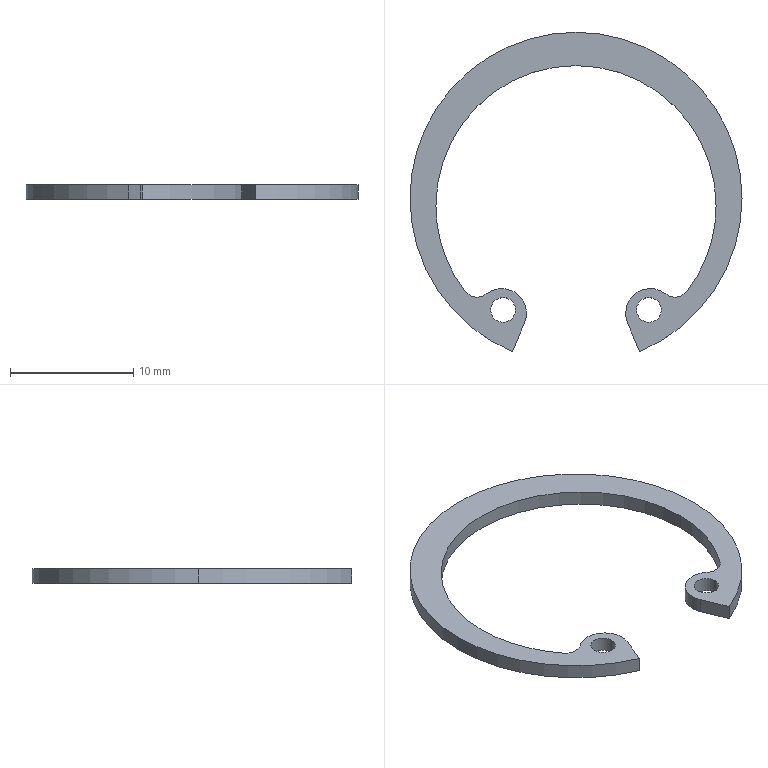Part | SolidWorks | features Extrusion 1 | 1 solid | 19 faces | box 26.9 x 25.876 x 1.2 mm | volume 193.596 mm3 | cylinder 15 | plane 4 | commonest cylinder face diameters 2 x4 4 x3 22.7 x3 26.9 x3 2.4 x2
STEP:
#1=CARTESIAN_POINT('',(4.909,-9.04,1.2));
#2=VERTEX_POINT('',#1);
#3=CARTESIAN_POINT('',(6.909,-9.04,1.2));
#4=VERTEX_POINT('',#3);
#5=CARTESIAN_POINT('',(5.909,-9.04,1.2));
#6=DIRECTION('',(0.,0.,1.));
#7=DIRECTION('',(-1.,0.,0.));
#8=AXIS2_PLACEMENT_3D('',#5,#6,#7);
#9=CIRCLE('',#8,1.);
#10=EDGE_CURVE('',#2,#4,#9,.T.);
#11=ORIENTED_EDGE('',*,*,#10,.T.);
#12=CARTESIAN_POINT('',(6.909,-9.04,0.));
#13=VERTEX_POINT('',#12);
#14=CARTESIAN_POINT('',(6.909,-9.04,1.2));
#15=DIRECTION('',(0.,0.,-1.));
#16=VECTOR('',#15,1000.);
#17=LINE('',#14,#16);
#18=EDGE_CURVE('',#4,#13,#17,.T.);
#19=ORIENTED_EDGE('',*,*,#18,.T.);
#20=CARTESIAN_POINT('',(4.909,-9.04,0.));
#21=VERTEX_POINT('',#20);
#22=CARTESIAN_POINT('',(5.909,-9.04,0.));
#23=DIRECTION('',(0.,0.,1.));
#24=DIRECTION('',(-1.,0.,0.));
#25=AXIS2_PLACEMENT_3D('',#22,#23,#24);
#26=CIRCLE('',#25,1.);
#27=EDGE_CURVE('',#21,#13,#26,.T.);
#28=ORIENTED_EDGE('',*,*,#27,.F.);
#29=CARTESIAN_POINT('',(4.909,-9.04,1.2));
#30=DIRECTION('',(0.,0.,-1.));
#31=VECTOR('',#30,1000.);
#32=LINE('',#29,#31);
#33=EDGE_CURVE('',#2,#21,#32,.T.);
#34=ORIENTED_EDGE('',*,*,#33,.F.);
#35=EDGE_LOOP('',(#11,#19,#28,#34));
#36=FACE_OUTER_BOUND('',#35,.T.);
#37=CARTESIAN_POINT('',(5.909,-9.04,1.2));
#38=DIRECTION('',(0.,0.,-1.));
#39=DIRECTION('',(-1.,0.,0.));
#40=AXIS2_PLACEMENT_3D('',#37,#38,#39);
#41=CYLINDRICAL_SURFACE('',#40,1.);
#42=ADVANCED_FACE('',(#36),#41,.F.);
#43=CARTESIAN_POINT('',(-6.909,-9.04,1.2));
#44=VERTEX_POINT('',#43);
#45=CARTESIAN_POINT('',(-4.909,-9.04,1.2));
#46=VERTEX_POINT('',#45);
#47=CARTESIAN_POINT('',(-5.909,-9.04,1.2));
#48=DIRECTION('',(0.,0.,1.));
#49=DIRECTION('',(1.,0.,0.));
#50=AXIS2_PLACEMENT_3D('',#47,#48,#49);
#51=CIRCLE('',#50,1.);
#52=EDGE_CURVE('',#44,#46,#51,.T.);
#53=ORIENTED_EDGE('',*,*,#52,.T.);
#54=CARTESIAN_POINT('',(-4.909,-9.04,0.));
#55=VERTEX_POINT('',#54);
#56=CARTESIAN_POINT('',(-4.909,-9.04,1.2));
#57=DIRECTION('',(0.,0.,-1.));
#58=VECTOR('',#57,1000.);
#59=LINE('',#56,#58);
#60=EDGE_CURVE('',#46,#55,#59,.T.);
#61=ORIENTED_EDGE('',*,*,#60,.T.);
#62=CARTESIAN_POINT('',(-6.909,-9.04,0.));
#63=VERTEX_POINT('',#62);
#64=CARTESIAN_POINT('',(-5.909,-9.04,0.));
#65=DIRECTION('',(0.,0.,1.));
#66=DIRECTION('',(1.,0.,0.));
#67=AXIS2_PLACEMENT_3D('',#64,#65,#66);
#68=CIRCLE('',#67,1.);
#69=EDGE_CURVE('',#63,#55,#68,.T.);
#70=ORIENTED_EDGE('',*,*,#69,.F.);
#71=CARTESIAN_POINT('',(-6.909,-9.04,1.2));
#72=DIRECTION('',(0.,0.,-1.));
#73=VECTOR('',#72,1000.);
#74=LINE('',#71,#73);
#75=EDGE_CURVE('',#44,#63,#74,.T.);
#76=ORIENTED_EDGE('',*,*,#75,.F.);
#77=EDGE_LOOP('',(#53,#61,#70,#76));
#78=FACE_OUTER_BOUND('',#77,.T.);
#79=CARTESIAN_POINT('',(-5.909,-9.04,1.2));
#80=DIRECTION('',(0.,0.,-1.));
#81=DIRECTION('',(-1.,0.,0.));
#82=AXIS2_PLACEMENT_3D('',#79,#80,#81);
#83=CYLINDRICAL_SURFACE('',#82,1.);
#84=ADVANCED_FACE('',(#78),#83,.F.);
#85=CARTESIAN_POINT('',(13.45,0.,1.2));
#86=VERTEX_POINT('',#85);
#87=CARTESIAN_POINT('',(-13.45,0.,1.2));
#88=VERTEX_POINT('',#87);
#89=CARTESIAN_POINT('',(0.,0.,1.2));
#90=DIRECTION('',(0.,0.,1.));
#91=DIRECTION('',(1.,0.,0.));
#92=AXIS2_PLACEMENT_3D('',#89,#90,#91);
#93=CIRCLE('',#92,13.45);
#94=EDGE_CURVE('',#86,#88,#93,.T.);
#95=ORIENTED_EDGE('',*,*,#94,.F.);
#96=CARTESIAN_POINT('',(13.45,0.,0.));
#97=VERTEX_POINT('',#96);
#98=CARTESIAN_POINT('',(13.45,0.,1.2));
#99=DIRECTION('',(0.,0.,-1.));
#100=VECTOR('',#99,1000.);
#101=LINE('',#98,#100);
#102=EDGE_CURVE('',#86,#97,#101,.T.);
#103=ORIENTED_EDGE('',*,*,#102,.T.);
#104=CARTESIAN_POINT('',(-13.45,0.,0.));
#105=VERTEX_POINT('',#104);
#106=CARTESIAN_POINT('',(0.,0.,0.));
#107=DIRECTION('',(0.,0.,1.));
#108=DIRECTION('',(1.,0.,0.));
#109=AXIS2_PLACEMENT_3D('',#106,#107,#108);
#110=CIRCLE('',#109,13.45);
#111=EDGE_CURVE('',#97,#105,#110,.T.);
#112=ORIENTED_EDGE('',*,*,#111,.T.);
#113=CARTESIAN_POINT('',(-13.45,0.,1.2));
#114=DIRECTION('',(0.,0.,-1.));
#115=VECTOR('',#114,1000.);
#116=LINE('',#113,#115);
#117=EDGE_CURVE('',#88,#105,#116,.T.);
#118=ORIENTED_EDGE('',*,*,#117,.F.);
#119=EDGE_LOOP('',(#95,#103,#112,#118));
#120=FACE_OUTER_BOUND('',#119,.T.);
#121=CARTESIAN_POINT('',(0.,0.,1.2));
#122=DIRECTION('',(0.,0.,-1.));
#123=DIRECTION('',(-1.,0.,0.));
#124=AXIS2_PLACEMENT_3D('',#121,#122,#123);
#125=CYLINDRICAL_SURFACE('',#124,13.45);
#126=ADVANCED_FACE('',(#120),#125,.T.);
#127=CARTESIAN_POINT('',(-5.147,-12.426,1.2));
#128=VERTEX_POINT('',#127);
#129=CARTESIAN_POINT('',(0.,0.,1.2));
#130=DIRECTION('',(0.,0.,1.));
#131=DIRECTION('',(1.,0.,0.));
#132=AXIS2_PLACEMENT_3D('',#129,#130,#131);
#133=CIRCLE('',#132,13.45);
#134=EDGE_CURVE('',#88,#128,#133,.T.);
#135=ORIENTED_EDGE('',*,*,#134,.F.);
#136=ORIENTED_EDGE('',*,*,#117,.T.);
#137=CARTESIAN_POINT('',(-5.147,-12.426,0.));
#138=VERTEX_POINT('',#137);
#139=CARTESIAN_POINT('',(0.,0.,0.));
#140=DIRECTION('',(0.,0.,1.));
#141=DIRECTION('',(1.,0.,0.));
#142=AXIS2_PLACEMENT_3D('',#139,#140,#141);
#143=CIRCLE('',#142,13.45);
#144=EDGE_CURVE('',#105,#138,#143,.T.);
#145=ORIENTED_EDGE('',*,*,#144,.T.);
#146=CARTESIAN_POINT('',(-5.147,-12.426,1.2));
#147=DIRECTION('',(0.,0.,-1.));
#148=VECTOR('',#147,1000.);
#149=LINE('',#146,#148);
#150=EDGE_CURVE('',#128,#138,#149,.T.);
#151=ORIENTED_EDGE('',*,*,#150,.F.);
#152=EDGE_LOOP('',(#135,#136,#145,#151));
#153=FACE_OUTER_BOUND('',#152,.T.);
#154=CARTESIAN_POINT('',(0.,0.,1.2));
#155=DIRECTION('',(0.,0.,-1.));
#156=DIRECTION('',(-1.,0.,0.));
#157=AXIS2_PLACEMENT_3D('',#154,#155,#156);
#158=CYLINDRICAL_SURFACE('',#157,13.45);
#159=ADVANCED_FACE('',(#153),#158,.T.);
#160=CARTESIAN_POINT('',(4.022,-9.312,1.2));
#161=VERTEX_POINT('',#160);
#162=CARTESIAN_POINT('',(4.174,-10.078,1.2));
#163=VERTEX_POINT('',#162);
#164=CARTESIAN_POINT('',(6.022,-9.312,1.2));
#165=DIRECTION('',(0.,0.,1.));
#166=DIRECTION('',(-1.,0.,0.));
#167=AXIS2_PLACEMENT_3D('',#164,#165,#166);
#168=CIRCLE('',#167,2.);
#169=EDGE_CURVE('',#161,#163,#168,.T.);
#170=ORIENTED_EDGE('',*,*,#169,.F.);
#171=CARTESIAN_POINT('',(4.022,-9.312,0.));
#172=VERTEX_POINT('',#171);
#173=CARTESIAN_POINT('',(4.022,-9.312,1.2));
#174=DIRECTION('',(0.,0.,-1.));
#175=VECTOR('',#174,1000.);
#176=LINE('',#173,#175);
#177=EDGE_CURVE('',#161,#172,#176,.T.);
#178=ORIENTED_EDGE('',*,*,#177,.T.);
#179=CARTESIAN_POINT('',(4.174,-10.078,0.));
#180=VERTEX_POINT('',#179);
#181=CARTESIAN_POINT('',(6.022,-9.312,0.));
#182=DIRECTION('',(0.,0.,1.));
#183=DIRECTION('',(-1.,0.,0.));
#184=AXIS2_PLACEMENT_3D('',#181,#182,#183);
#185=CIRCLE('',#184,2.);
#186=EDGE_CURVE('',#172,#180,#185,.T.);
#187=ORIENTED_EDGE('',*,*,#186,.T.);
#188=CARTESIAN_POINT('',(4.174,-10.078,1.2));
#189=DIRECTION('',(0.,0.,-1.));
#190=VECTOR('',#189,1000.);
#191=LINE('',#188,#190);
#192=EDGE_CURVE('',#163,#180,#191,.T.);
#193=ORIENTED_EDGE('',*,*,#192,.F.);
#194=EDGE_LOOP('',(#170,#178,#187,#193));
#195=FACE_OUTER_BOUND('',#194,.T.);
#196=CARTESIAN_POINT('',(6.022,-9.312,1.2));
#197=DIRECTION('',(0.,0.,-1.));
#198=DIRECTION('',(-1.,0.,0.));
#199=AXIS2_PLACEMENT_3D('',#196,#197,#198);
#200=CYLINDRICAL_SURFACE('',#199,2.);
#201=ADVANCED_FACE('',(#195),#200,.T.);
#202=CARTESIAN_POINT('',(11.35,-0.6,1.2));
#203=VERTEX_POINT('',#202);
#204=CARTESIAN_POINT('',(8.973,-7.551,1.2));
#205=VERTEX_POINT('',#204);
#206=CARTESIAN_POINT('',(0.,-0.6,1.2));
#207=DIRECTION('',(0.,0.,-1.));
#208=DIRECTION('',(1.,0.,0.));
#209=AXIS2_PLACEMENT_3D('',#206,#207,#208);
#210=CIRCLE('',#209,11.35);
#211=EDGE_CURVE('',#203,#205,#210,.T.);
#212=ORIENTED_EDGE('',*,*,#211,.F.);
#213=CARTESIAN_POINT('',(11.35,-0.6,0.));
#214=VERTEX_POINT('',#213);
#215=CARTESIAN_POINT('',(11.35,-0.6,1.2));
#216=DIRECTION('',(0.,0.,-1.));
#217=VECTOR('',#216,1000.);
#218=LINE('',#215,#217);
#219=EDGE_CURVE('',#203,#214,#218,.T.);
#220=ORIENTED_EDGE('',*,*,#219,.T.);
#221=CARTESIAN_POINT('',(8.973,-7.551,0.));
#222=VERTEX_POINT('',#221);
#223=CARTESIAN_POINT('',(0.,-0.6,0.));
#224=DIRECTION('',(0.,0.,-1.));
#225=DIRECTION('',(1.,0.,0.));
#226=AXIS2_PLACEMENT_3D('',#223,#224,#225);
#227=CIRCLE('',#226,11.35);
#228=EDGE_CURVE('',#214,#222,#227,.T.);
#229=ORIENTED_EDGE('',*,*,#228,.T.);
#230=CARTESIAN_POINT('',(8.973,-7.551,1.2));
#231=DIRECTION('',(0.,0.,-1.));
#232=VECTOR('',#231,1000.);
#233=LINE('',#230,#232);
#234=EDGE_CURVE('',#205,#222,#233,.T.);
#235=ORIENTED_EDGE('',*,*,#234,.F.);
#236=EDGE_LOOP('',(#212,#220,#229,#235));
#237=FACE_OUTER_BOUND('',#236,.T.);
#238=CARTESIAN_POINT('',(0.,-0.6,1.2));
#239=DIRECTION('',(0.,0.,-1.));
#240=DIRECTION('',(-1.,0.,0.));
#241=AXIS2_PLACEMENT_3D('',#238,#239,#240);
#242=CYLINDRICAL_SURFACE('',#241,11.35);
#243=ADVANCED_FACE('',(#237),#242,.F.);
#244=ORIENTED_EDGE('',*,*,#219,.F.);
#245=CARTESIAN_POINT('',(-11.35,-0.6,1.2));
#246=VERTEX_POINT('',#245);
#247=CARTESIAN_POINT('',(0.,-0.6,1.2));
#248=DIRECTION('',(0.,0.,-1.));
#249=DIRECTION('',(1.,0.,0.));
#250=AXIS2_PLACEMENT_3D('',#247,#248,#249);
#251=CIRCLE('',#250,11.35);
#252=EDGE_CURVE('',#246,#203,#251,.T.);
#253=ORIENTED_EDGE('',*,*,#252,.F.);
#254=CARTESIAN_POINT('',(-11.35,-0.6,0.));
#255=VERTEX_POINT('',#254);
#256=CARTESIAN_POINT('',(-11.35,-0.6,1.2));
#257=DIRECTION('',(0.,0.,-1.));
#258=VECTOR('',#257,1000.);
#259=LINE('',#256,#258);
#260=EDGE_CURVE('',#246,#255,#259,.T.);
#261=ORIENTED_EDGE('',*,*,#260,.T.);
#262=CARTESIAN_POINT('',(0.,-0.6,0.));
#263=DIRECTION('',(0.,0.,-1.));
#264=DIRECTION('',(1.,0.,0.));
#265=AXIS2_PLACEMENT_3D('',#262,#263,#264);
#266=CIRCLE('',#265,11.35);
#267=EDGE_CURVE('',#255,#214,#266,.T.);
#268=ORIENTED_EDGE('',*,*,#267,.T.);
#269=EDGE_LOOP('',(#244,#253,#261,#268));
#270=FACE_OUTER_BOUND('',#269,.T.);
#271=CARTESIAN_POINT('',(0.,-0.6,1.2));
#272=DIRECTION('',(0.,0.,-1.));
#273=DIRECTION('',(-1.,0.,0.));
#274=AXIS2_PLACEMENT_3D('',#271,#272,#273);
#275=CYLINDRICAL_SURFACE('',#274,11.35);
#276=ADVANCED_FACE('',(#270),#275,.F.);
#277=ORIENTED_EDGE('',*,*,#52,.F.);
#278=CARTESIAN_POINT('',(-5.909,-9.04,1.2));
#279=DIRECTION('',(0.,0.,1.));
#280=DIRECTION('',(1.,0.,0.));
#281=AXIS2_PLACEMENT_3D('',#278,#279,#280);
#282=CIRCLE('',#281,1.);
#283=EDGE_CURVE('',#46,#44,#282,.T.);
#284=ORIENTED_EDGE('',*,*,#283,.F.);
#285=EDGE_LOOP('',(#277,#284));
#286=FACE_BOUND('',#285,.T.);
#287=CARTESIAN_POINT('',(-4.174,-10.078,1.2));
#288=VERTEX_POINT('',#287);
#289=CARTESIAN_POINT('',(-7.273,-7.752,1.2));
#290=VERTEX_POINT('',#289);
#291=CARTESIAN_POINT('',(-6.022,-9.312,1.2));
#292=DIRECTION('',(0.,0.,1.));
#293=DIRECTION('',(1.,0.,0.));
#294=AXIS2_PLACEMENT_3D('',#291,#292,#293);
#295=CIRCLE('',#294,2.);
#296=EDGE_CURVE('',#288,#290,#295,.T.);
#297=ORIENTED_EDGE('',*,*,#296,.T.);
#298=CARTESIAN_POINT('',(-8.973,-7.551,1.2));
#299=VERTEX_POINT('',#298);
#300=CARTESIAN_POINT('',(-8.024,-6.816,1.2));
#301=DIRECTION('',(0.,0.,-1.));
#302=DIRECTION('',(-1.,0.,0.));
#303=AXIS2_PLACEMENT_3D('',#300,#301,#302);
#304=CIRCLE('',#303,1.2);
#305=EDGE_CURVE('',#290,#299,#304,.T.);
#306=ORIENTED_EDGE('',*,*,#305,.T.);
#307=CARTESIAN_POINT('',(0.,-0.6,1.2));
#308=DIRECTION('',(0.,0.,-1.));
#309=DIRECTION('',(1.,0.,0.));
#310=AXIS2_PLACEMENT_3D('',#307,#308,#309);
#311=CIRCLE('',#310,11.35);
#312=EDGE_CURVE('',#299,#246,#311,.T.);
#313=ORIENTED_EDGE('',*,*,#312,.T.);
#314=ORIENTED_EDGE('',*,*,#252,.T.);
#315=ORIENTED_EDGE('',*,*,#211,.T.);
#316=CARTESIAN_POINT('',(7.273,-7.752,1.2));
#317=VERTEX_POINT('',#316);
#318=CARTESIAN_POINT('',(8.024,-6.816,1.2));
#319=DIRECTION('',(0.,0.,-1.));
#320=DIRECTION('',(1.,0.,0.));
#321=AXIS2_PLACEMENT_3D('',#318,#319,#320);
#322=CIRCLE('',#321,1.2);
#323=EDGE_CURVE('',#205,#317,#322,.T.);
#324=ORIENTED_EDGE('',*,*,#323,.T.);
#325=CARTESIAN_POINT('',(6.022,-9.312,1.2));
#326=DIRECTION('',(0.,0.,1.));
#327=DIRECTION('',(-1.,0.,0.));
#328=AXIS2_PLACEMENT_3D('',#325,#326,#327);
#329=CIRCLE('',#328,2.);
#330=EDGE_CURVE('',#317,#161,#329,.T.);
#331=ORIENTED_EDGE('',*,*,#330,.T.);
#332=ORIENTED_EDGE('',*,*,#169,.T.);
#333=CARTESIAN_POINT('',(5.147,-12.426,1.2));
#334=VERTEX_POINT('',#333);
#335=CARTESIAN_POINT('',(4.174,-10.078,1.2));
#336=DIRECTION('',(0.3827,-0.9239,0.));
#337=VECTOR('',#336,1000.);
#338=LINE('',#335,#337);
#339=EDGE_CURVE('',#163,#334,#338,.T.);
#340=ORIENTED_EDGE('',*,*,#339,.T.);
#341=CARTESIAN_POINT('',(0.,0.,1.2));
#342=DIRECTION('',(0.,0.,1.));
#343=DIRECTION('',(1.,0.,0.));
#344=AXIS2_PLACEMENT_3D('',#341,#342,#343);
#345=CIRCLE('',#344,13.45);
#346=EDGE_CURVE('',#334,#86,#345,.T.);
#347=ORIENTED_EDGE('',*,*,#346,.T.);
#348=ORIENTED_EDGE('',*,*,#94,.T.);
#349=ORIENTED_EDGE('',*,*,#134,.T.);
#350=CARTESIAN_POINT('',(-4.174,-10.078,1.2));
#351=DIRECTION('',(0.3827,0.9239,0.));
#352=VECTOR('',#351,1000.);
#353=LINE('',#350,#352);
#354=EDGE_CURVE('',#128,#288,#353,.T.);
#355=ORIENTED_EDGE('',*,*,#354,.T.);
#356=EDGE_LOOP('',(#297,#306,#313,#314,#315,#324,#331,#332,#340,#347,#348,#349,#355));
#357=FACE_OUTER_BOUND('',#356,.T.);
#358=ORIENTED_EDGE('',*,*,#10,.F.);
#359=CARTESIAN_POINT('',(5.909,-9.04,1.2));
#360=DIRECTION('',(0.,0.,1.));
#361=DIRECTION('',(-1.,0.,0.));
#362=AXIS2_PLACEMENT_3D('',#359,#360,#361);
#363=CIRCLE('',#362,1.);
#364=EDGE_CURVE('',#4,#2,#363,.T.);
#365=ORIENTED_EDGE('',*,*,#364,.F.);
#366=EDGE_LOOP('',(#358,#365));
#367=FACE_BOUND('',#366,.T.);
#368=CARTESIAN_POINT('',(-6.022,-9.312,1.2));
#369=DIRECTION('',(0.,0.,1.));
#370=DIRECTION('',(1.,0.,0.));
#371=AXIS2_PLACEMENT_3D('',#368,#369,#370);
#372=PLANE('',#371);
#373=ADVANCED_FACE('',(#286,#357,#367),#372,.T.);
#374=CARTESIAN_POINT('',(-4.174,-10.078,0.));
#375=VERTEX_POINT('',#374);
#376=CARTESIAN_POINT('',(-7.273,-7.752,0.));
#377=VERTEX_POINT('',#376);
#378=CARTESIAN_POINT('',(-6.022,-9.312,0.));
#379=DIRECTION('',(0.,0.,1.));
#380=DIRECTION('',(1.,0.,0.));
#381=AXIS2_PLACEMENT_3D('',#378,#379,#380);
#382=CIRCLE('',#381,2.);
#383=EDGE_CURVE('',#375,#377,#382,.T.);
#384=ORIENTED_EDGE('',*,*,#383,.F.);
#385=CARTESIAN_POINT('',(-4.174,-10.078,0.));
#386=DIRECTION('',(0.3827,0.9239,0.));
#387=VECTOR('',#386,1000.);
#388=LINE('',#385,#387);
#389=EDGE_CURVE('',#138,#375,#388,.T.);
#390=ORIENTED_EDGE('',*,*,#389,.F.);
#391=ORIENTED_EDGE('',*,*,#144,.F.);
#392=ORIENTED_EDGE('',*,*,#111,.F.);
#393=CARTESIAN_POINT('',(5.147,-12.426,0.));
#394=VERTEX_POINT('',#393);
#395=CARTESIAN_POINT('',(0.,0.,0.));
#396=DIRECTION('',(0.,0.,1.));
#397=DIRECTION('',(1.,0.,0.));
#398=AXIS2_PLACEMENT_3D('',#395,#396,#397);
#399=CIRCLE('',#398,13.45);
#400=EDGE_CURVE('',#394,#97,#399,.T.);
#401=ORIENTED_EDGE('',*,*,#400,.F.);
#402=CARTESIAN_POINT('',(4.174,-10.078,0.));
#403=DIRECTION('',(0.3827,-0.9239,0.));
#404=VECTOR('',#403,1000.);
#405=LINE('',#402,#404);
#406=EDGE_CURVE('',#180,#394,#405,.T.);
#407=ORIENTED_EDGE('',*,*,#406,.F.);
#408=ORIENTED_EDGE('',*,*,#186,.F.);
#409=CARTESIAN_POINT('',(7.273,-7.752,0.));
#410=VERTEX_POINT('',#409);
#411=CARTESIAN_POINT('',(6.022,-9.312,0.));
#412=DIRECTION('',(0.,0.,1.));
#413=DIRECTION('',(-1.,0.,0.));
#414=AXIS2_PLACEMENT_3D('',#411,#412,#413);
#415=CIRCLE('',#414,2.);
#416=EDGE_CURVE('',#410,#172,#415,.T.);
#417=ORIENTED_EDGE('',*,*,#416,.F.);
#418=CARTESIAN_POINT('',(8.024,-6.816,0.));
#419=DIRECTION('',(0.,0.,-1.));
#420=DIRECTION('',(1.,0.,0.));
#421=AXIS2_PLACEMENT_3D('',#418,#419,#420);
#422=CIRCLE('',#421,1.2);
#423=EDGE_CURVE('',#222,#410,#422,.T.);
#424=ORIENTED_EDGE('',*,*,#423,.F.);
#425=ORIENTED_EDGE('',*,*,#228,.F.);
#426=ORIENTED_EDGE('',*,*,#267,.F.);
#427=CARTESIAN_POINT('',(-8.973,-7.551,0.));
#428=VERTEX_POINT('',#427);
#429=CARTESIAN_POINT('',(0.,-0.6,0.));
#430=DIRECTION('',(0.,0.,-1.));
#431=DIRECTION('',(1.,0.,0.));
#432=AXIS2_PLACEMENT_3D('',#429,#430,#431);
#433=CIRCLE('',#432,11.35);
#434=EDGE_CURVE('',#428,#255,#433,.T.);
#435=ORIENTED_EDGE('',*,*,#434,.F.);
#436=CARTESIAN_POINT('',(-8.024,-6.816,0.));
#437=DIRECTION('',(0.,0.,-1.));
#438=DIRECTION('',(-1.,0.,0.));
#439=AXIS2_PLACEMENT_3D('',#436,#437,#438);
#440=CIRCLE('',#439,1.2);
#441=EDGE_CURVE('',#377,#428,#440,.T.);
#442=ORIENTED_EDGE('',*,*,#441,.F.);
#443=EDGE_LOOP('',(#384,#390,#391,#392,#401,#407,#408,#417,#424,#425,#426,#435,#442));
#444=FACE_OUTER_BOUND('',#443,.T.);
#445=ORIENTED_EDGE('',*,*,#69,.T.);
#446=CARTESIAN_POINT('',(-5.909,-9.04,0.));
#447=DIRECTION('',(0.,0.,1.));
#448=DIRECTION('',(1.,0.,0.));
#449=AXIS2_PLACEMENT_3D('',#446,#447,#448);
#450=CIRCLE('',#449,1.);
#451=EDGE_CURVE('',#55,#63,#450,.T.);
#452=ORIENTED_EDGE('',*,*,#451,.T.);
#453=EDGE_LOOP('',(#445,#452));
#454=FACE_BOUND('',#453,.T.);
#455=ORIENTED_EDGE('',*,*,#27,.T.);
#456=CARTESIAN_POINT('',(5.909,-9.04,0.));
#457=DIRECTION('',(0.,0.,1.));
#458=DIRECTION('',(-1.,0.,0.));
#459=AXIS2_PLACEMENT_3D('',#456,#457,#458);
#460=CIRCLE('',#459,1.);
#461=EDGE_CURVE('',#13,#21,#460,.T.);
#462=ORIENTED_EDGE('',*,*,#461,.T.);
#463=EDGE_LOOP('',(#455,#462));
#464=FACE_BOUND('',#463,.T.);
#465=CARTESIAN_POINT('',(-6.022,-9.312,0.));
#466=DIRECTION('',(0.,0.,1.));
#467=DIRECTION('',(1.,0.,0.));
#468=AXIS2_PLACEMENT_3D('',#465,#466,#467);
#469=PLANE('',#468);
#470=ADVANCED_FACE('',(#444,#454,#464),#469,.F.);
#471=ORIENTED_EDGE('',*,*,#383,.T.);
#472=CARTESIAN_POINT('',(-7.273,-7.752,1.2));
#473=DIRECTION('',(0.,0.,-1.));
#474=VECTOR('',#473,1000.);
#475=LINE('',#472,#474);
#476=EDGE_CURVE('',#290,#377,#475,.T.);
#477=ORIENTED_EDGE('',*,*,#476,.F.);
#478=ORIENTED_EDGE('',*,*,#296,.F.);
#479=CARTESIAN_POINT('',(-4.174,-10.078,1.2));
#480=DIRECTION('',(0.,0.,-1.));
#481=VECTOR('',#480,1000.);
#482=LINE('',#479,#481);
#483=EDGE_CURVE('',#288,#375,#482,.T.);
#484=ORIENTED_EDGE('',*,*,#483,.T.);
#485=EDGE_LOOP('',(#471,#477,#478,#484));
#486=FACE_OUTER_BOUND('',#485,.T.);
#487=CARTESIAN_POINT('',(-6.022,-9.312,1.2));
#488=DIRECTION('',(0.,0.,-1.));
#489=DIRECTION('',(-1.,0.,0.));
#490=AXIS2_PLACEMENT_3D('',#487,#488,#489);
#491=CYLINDRICAL_SURFACE('',#490,2.);
#492=ADVANCED_FACE('',(#486),#491,.T.);
#493=ORIENTED_EDGE('',*,*,#441,.T.);
#494=CARTESIAN_POINT('',(-8.973,-7.551,1.2));
#495=DIRECTION('',(0.,0.,-1.));
#496=VECTOR('',#495,1000.);
#497=LINE('',#494,#496);
#498=EDGE_CURVE('',#299,#428,#497,.T.);
#499=ORIENTED_EDGE('',*,*,#498,.F.);
#500=ORIENTED_EDGE('',*,*,#305,.F.);
#501=ORIENTED_EDGE('',*,*,#476,.T.);
#502=EDGE_LOOP('',(#493,#499,#500,#501));
#503=FACE_OUTER_BOUND('',#502,.T.);
#504=CARTESIAN_POINT('',(-8.024,-6.816,1.2));
#505=DIRECTION('',(0.,0.,-1.));
#506=DIRECTION('',(-1.,0.,0.));
#507=AXIS2_PLACEMENT_3D('',#504,#505,#506);
#508=CYLINDRICAL_SURFACE('',#507,1.2);
#509=ADVANCED_FACE('',(#503),#508,.F.);
#510=ORIENTED_EDGE('',*,*,#260,.F.);
#511=ORIENTED_EDGE('',*,*,#312,.F.);
#512=ORIENTED_EDGE('',*,*,#498,.T.);
#513=ORIENTED_EDGE('',*,*,#434,.T.);
#514=EDGE_LOOP('',(#510,#511,#512,#513));
#515=FACE_OUTER_BOUND('',#514,.T.);
#516=CARTESIAN_POINT('',(0.,-0.6,1.2));
#517=DIRECTION('',(0.,0.,-1.));
#518=DIRECTION('',(-1.,0.,0.));
#519=AXIS2_PLACEMENT_3D('',#516,#517,#518);
#520=CYLINDRICAL_SURFACE('',#519,11.35);
#521=ADVANCED_FACE('',(#515),#520,.F.);
#522=ORIENTED_EDGE('',*,*,#423,.T.);
#523=CARTESIAN_POINT('',(7.273,-7.752,1.2));
#524=DIRECTION('',(0.,0.,-1.));
#525=VECTOR('',#524,1000.);
#526=LINE('',#523,#525);
#527=EDGE_CURVE('',#317,#410,#526,.T.);
#528=ORIENTED_EDGE('',*,*,#527,.F.);
#529=ORIENTED_EDGE('',*,*,#323,.F.);
#530=ORIENTED_EDGE('',*,*,#234,.T.);
#531=EDGE_LOOP('',(#522,#528,#529,#530));
#532=FACE_OUTER_BOUND('',#531,.T.);
#533=CARTESIAN_POINT('',(8.024,-6.816,1.2));
#534=DIRECTION('',(0.,0.,-1.));
#535=DIRECTION('',(-1.,0.,0.));
#536=AXIS2_PLACEMENT_3D('',#533,#534,#535);
#537=CYLINDRICAL_SURFACE('',#536,1.2);
#538=ADVANCED_FACE('',(#532),#537,.F.);
#539=ORIENTED_EDGE('',*,*,#177,.F.);
#540=ORIENTED_EDGE('',*,*,#330,.F.);
#541=ORIENTED_EDGE('',*,*,#527,.T.);
#542=ORIENTED_EDGE('',*,*,#416,.T.);
#543=EDGE_LOOP('',(#539,#540,#541,#542));
#544=FACE_OUTER_BOUND('',#543,.T.);
#545=CARTESIAN_POINT('',(6.022,-9.312,1.2));
#546=DIRECTION('',(0.,0.,-1.));
#547=DIRECTION('',(-1.,0.,0.));
#548=AXIS2_PLACEMENT_3D('',#545,#546,#547);
#549=CYLINDRICAL_SURFACE('',#548,2.);
#550=ADVANCED_FACE('',(#544),#549,.T.);
#551=ORIENTED_EDGE('',*,*,#406,.T.);
#552=CARTESIAN_POINT('',(5.147,-12.426,1.2));
#553=DIRECTION('',(0.,0.,-1.));
#554=VECTOR('',#553,1000.);
#555=LINE('',#552,#554);
#556=EDGE_CURVE('',#334,#394,#555,.T.);
#557=ORIENTED_EDGE('',*,*,#556,.F.);
#558=ORIENTED_EDGE('',*,*,#339,.F.);
#559=ORIENTED_EDGE('',*,*,#192,.T.);
#560=EDGE_LOOP('',(#551,#557,#558,#559));
#561=FACE_OUTER_BOUND('',#560,.T.);
#562=CARTESIAN_POINT('',(4.174,-10.078,1.2));
#563=DIRECTION('',(0.9239,0.3827,0.));
#564=DIRECTION('',(-0.3827,0.9239,0.));
#565=AXIS2_PLACEMENT_3D('',#562,#563,#564);
#566=PLANE('',#565);
#567=ADVANCED_FACE('',(#561),#566,.F.);
#568=ORIENTED_EDGE('',*,*,#102,.F.);
#569=ORIENTED_EDGE('',*,*,#346,.F.);
#570=ORIENTED_EDGE('',*,*,#556,.T.);
#571=ORIENTED_EDGE('',*,*,#400,.T.);
#572=EDGE_LOOP('',(#568,#569,#570,#571));
#573=FACE_OUTER_BOUND('',#572,.T.);
#574=CARTESIAN_POINT('',(0.,0.,1.2));
#575=DIRECTION('',(0.,0.,-1.));
#576=DIRECTION('',(-1.,0.,0.));
#577=AXIS2_PLACEMENT_3D('',#574,#575,#576);
#578=CYLINDRICAL_SURFACE('',#577,13.45);
#579=ADVANCED_FACE('',(#573),#578,.T.);
#580=ORIENTED_EDGE('',*,*,#389,.T.);
#581=ORIENTED_EDGE('',*,*,#483,.F.);
#582=ORIENTED_EDGE('',*,*,#354,.F.);
#583=ORIENTED_EDGE('',*,*,#150,.T.);
#584=EDGE_LOOP('',(#580,#581,#582,#583));
#585=FACE_OUTER_BOUND('',#584,.T.);
#586=CARTESIAN_POINT('',(-4.174,-10.078,1.2));
#587=DIRECTION('',(-0.9239,0.3827,0.));
#588=DIRECTION('',(-0.3827,-0.9239,0.));
#589=AXIS2_PLACEMENT_3D('',#586,#587,#588);
#590=PLANE('',#589);
#591=ADVANCED_FACE('',(#585),#590,.F.);
#592=ORIENTED_EDGE('',*,*,#60,.F.);
#593=ORIENTED_EDGE('',*,*,#283,.T.);
#594=ORIENTED_EDGE('',*,*,#75,.T.);
#595=ORIENTED_EDGE('',*,*,#451,.F.);
#596=EDGE_LOOP('',(#592,#593,#594,#595));
#597=FACE_OUTER_BOUND('',#596,.T.);
#598=CARTESIAN_POINT('',(-5.909,-9.04,1.2));
#599=DIRECTION('',(0.,0.,-1.));
#600=DIRECTION('',(-1.,0.,0.));
#601=AXIS2_PLACEMENT_3D('',#598,#599,#600);
#602=CYLINDRICAL_SURFACE('',#601,1.);
#603=ADVANCED_FACE('',(#597),#602,.F.);
#604=ORIENTED_EDGE('',*,*,#18,.F.);
#605=ORIENTED_EDGE('',*,*,#364,.T.);
#606=ORIENTED_EDGE('',*,*,#33,.T.);
#607=ORIENTED_EDGE('',*,*,#461,.F.);
#608=EDGE_LOOP('',(#604,#605,#606,#607));
#609=FACE_OUTER_BOUND('',#608,.T.);
#610=CARTESIAN_POINT('',(5.909,-9.04,1.2));
#611=DIRECTION('',(0.,0.,-1.));
#612=DIRECTION('',(-1.,0.,0.));
#613=AXIS2_PLACEMENT_3D('',#610,#611,#612);
#614=CYLINDRICAL_SURFACE('',#613,1.);
#615=ADVANCED_FACE('',(#609),#614,.F.);
#616=CLOSED_SHELL('',(#42,#84,#126,#159,#201,#243,#276,#373,#470,#492,#509,#521,#538,#550,#567,#579,#591,#603,#615));
#617=MANIFOLD_SOLID_BREP('',#616);
#618=CARTESIAN_POINT('',(0.,0.,0.));
#619=DIRECTION('',(0.,0.,1.));
#620=DIRECTION('',(1.,0.,0.));
#621=AXIS2_PLACEMENT_3D('',#618,#619,#620);
#622=(LENGTH_UNIT()NAMED_UNIT(*)SI_UNIT(.MILLI.,.METRE.));
#623=UNCERTAINTY_MEASURE_WITH_UNIT(LENGTH_MEASURE(0.00001),#622,'','');
#624=(NAMED_UNIT(*)PLANE_ANGLE_UNIT()SI_UNIT($,.RADIAN.));
#625=(NAMED_UNIT(*)SI_UNIT($,.STERADIAN.)SOLID_ANGLE_UNIT());
#626=(GEOMETRIC_REPRESENTATION_CONTEXT(3)GLOBAL_UNCERTAINTY_ASSIGNED_CONTEXT((#623))GLOBAL_UNIT_ASSIGNED_CONTEXT((#622,#624,#625))REPRESENTATION_CONTEXT('',''));
#627=ADVANCED_BREP_SHAPE_REPRESENTATION('',(#617,#621),#626);